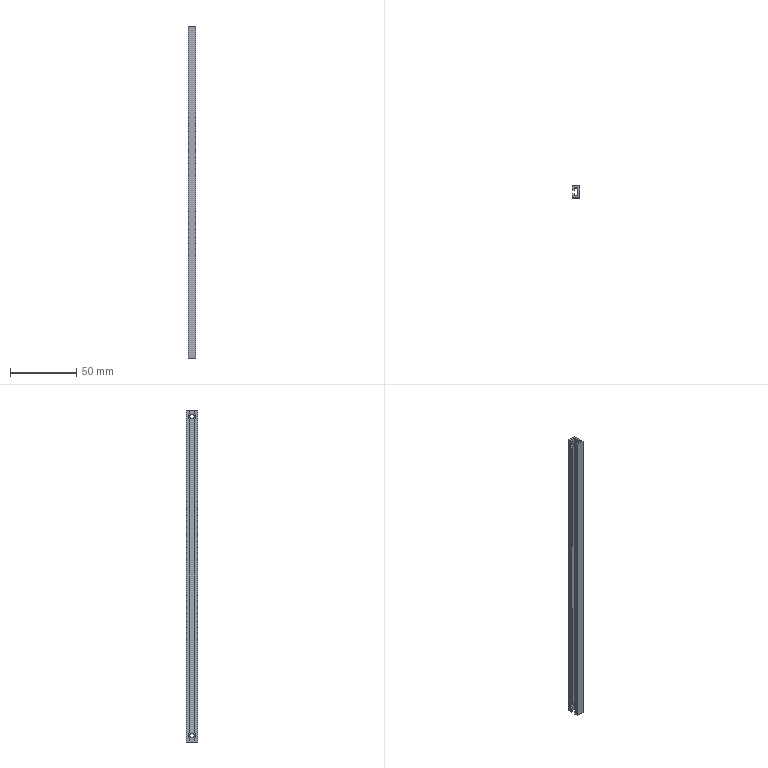Part | SolidWorks | features Extrusion 1, HoleWzd 1 | 1 solid | 34 faces | box 6 x 9 x 250 mm | volume 7894 mm3 | plane 26 | cylinder 8 | commonest cylinder face diameters 3.4 x4 6 x4
STEP:
#1=CARTESIAN_POINT('',(3.,0.,243.3));
#2=VERTEX_POINT('',#1);
#3=CARTESIAN_POINT('',(3.,0.,246.7));
#4=VERTEX_POINT('',#3);
#5=CARTESIAN_POINT('',(3.,0.,245.));
#6=DIRECTION('',(-1.,0.,0.));
#7=DIRECTION('',(0.,0.,1.));
#8=AXIS2_PLACEMENT_3D('',#5,#6,#7);
#9=CIRCLE('',#8,1.7);
#10=EDGE_CURVE('',#2,#4,#9,.T.);
#11=ORIENTED_EDGE('',*,*,#10,.F.);
#12=CARTESIAN_POINT('',(1.5,0.,243.3));
#13=VERTEX_POINT('',#12);
#14=CARTESIAN_POINT('',(-3.,0.,243.3));
#15=DIRECTION('',(-1.,0.,0.));
#16=VECTOR('',#15,1000.);
#17=LINE('',#14,#16);
#18=EDGE_CURVE('',#2,#13,#17,.T.);
#19=ORIENTED_EDGE('',*,*,#18,.T.);
#20=CARTESIAN_POINT('',(1.5,0.,246.7));
#21=VERTEX_POINT('',#20);
#22=CARTESIAN_POINT('',(1.5,0.,245.));
#23=DIRECTION('',(1.,0.,0.));
#24=DIRECTION('',(0.,0.,-1.));
#25=AXIS2_PLACEMENT_3D('',#22,#23,#24);
#26=CIRCLE('',#25,1.7);
#27=EDGE_CURVE('',#21,#13,#26,.T.);
#28=ORIENTED_EDGE('',*,*,#27,.F.);
#29=CARTESIAN_POINT('',(-3.,0.,246.7));
#30=DIRECTION('',(-1.,0.,0.));
#31=VECTOR('',#30,1000.);
#32=LINE('',#29,#31);
#33=EDGE_CURVE('',#4,#21,#32,.T.);
#34=ORIENTED_EDGE('',*,*,#33,.F.);
#35=EDGE_LOOP('',(#11,#19,#28,#34));
#36=FACE_OUTER_BOUND('',#35,.T.);
#37=CARTESIAN_POINT('',(-3.,0.,245.));
#38=DIRECTION('',(-1.,0.,0.));
#39=DIRECTION('',(0.,0.,1.));
#40=AXIS2_PLACEMENT_3D('',#37,#38,#39);
#41=CYLINDRICAL_SURFACE('',#40,1.7);
#42=ADVANCED_FACE('',(#36),#41,.F.);
#43=CARTESIAN_POINT('',(3.,0.,3.3));
#44=VERTEX_POINT('',#43);
#45=CARTESIAN_POINT('',(3.,0.,6.7));
#46=VERTEX_POINT('',#45);
#47=CARTESIAN_POINT('',(3.,0.,5.));
#48=DIRECTION('',(-1.,0.,0.));
#49=DIRECTION('',(0.,0.,1.));
#50=AXIS2_PLACEMENT_3D('',#47,#48,#49);
#51=CIRCLE('',#50,1.7);
#52=EDGE_CURVE('',#44,#46,#51,.T.);
#53=ORIENTED_EDGE('',*,*,#52,.F.);
#54=CARTESIAN_POINT('',(1.5,0.,3.3));
#55=VERTEX_POINT('',#54);
#56=CARTESIAN_POINT('',(-3.,0.,3.3));
#57=DIRECTION('',(-1.,0.,0.));
#58=VECTOR('',#57,1000.);
#59=LINE('',#56,#58);
#60=EDGE_CURVE('',#44,#55,#59,.T.);
#61=ORIENTED_EDGE('',*,*,#60,.T.);
#62=CARTESIAN_POINT('',(1.5,0.,6.7));
#63=VERTEX_POINT('',#62);
#64=CARTESIAN_POINT('',(1.5,0.,5.));
#65=DIRECTION('',(1.,0.,0.));
#66=DIRECTION('',(0.,0.,-1.));
#67=AXIS2_PLACEMENT_3D('',#64,#65,#66);
#68=CIRCLE('',#67,1.7);
#69=EDGE_CURVE('',#63,#55,#68,.T.);
#70=ORIENTED_EDGE('',*,*,#69,.F.);
#71=CARTESIAN_POINT('',(-3.,0.,6.7));
#72=DIRECTION('',(-1.,0.,0.));
#73=VECTOR('',#72,1000.);
#74=LINE('',#71,#73);
#75=EDGE_CURVE('',#46,#63,#74,.T.);
#76=ORIENTED_EDGE('',*,*,#75,.F.);
#77=EDGE_LOOP('',(#53,#61,#70,#76));
#78=FACE_OUTER_BOUND('',#77,.T.);
#79=CARTESIAN_POINT('',(-3.,0.,5.));
#80=DIRECTION('',(-1.,0.,0.));
#81=DIRECTION('',(0.,0.,1.));
#82=AXIS2_PLACEMENT_3D('',#79,#80,#81);
#83=CYLINDRICAL_SURFACE('',#82,1.7);
#84=ADVANCED_FACE('',(#78),#83,.F.);
#85=CARTESIAN_POINT('',(-1.5,1.7,250.));
#86=VERTEX_POINT('',#85);
#87=CARTESIAN_POINT('',(-1.5,1.7,247.472));
#88=VERTEX_POINT('',#87);
#89=CARTESIAN_POINT('',(-1.5,1.7,250.));
#90=DIRECTION('',(0.,0.,-1.));
#91=VECTOR('',#90,1000.);
#92=LINE('',#89,#91);
#93=EDGE_CURVE('',#86,#88,#92,.T.);
#94=ORIENTED_EDGE('',*,*,#93,.T.);
#95=CARTESIAN_POINT('',(-1.5,2.85,245.937));
#96=VERTEX_POINT('',#95);
#97=CARTESIAN_POINT('',(-1.5,0.,245.));
#98=DIRECTION('',(-1.,0.,0.));
#99=DIRECTION('',(0.,0.,1.));
#100=AXIS2_PLACEMENT_3D('',#97,#98,#99);
#101=CIRCLE('',#100,3.);
#102=EDGE_CURVE('',#88,#96,#101,.T.);
#103=ORIENTED_EDGE('',*,*,#102,.T.);
#104=CARTESIAN_POINT('',(-1.5,2.85,250.));
#105=VERTEX_POINT('',#104);
#106=CARTESIAN_POINT('',(-1.5,2.85,250.));
#107=DIRECTION('',(0.,0.,-1.));
#108=VECTOR('',#107,1000.);
#109=LINE('',#106,#108);
#110=EDGE_CURVE('',#105,#96,#109,.T.);
#111=ORIENTED_EDGE('',*,*,#110,.F.);
#112=CARTESIAN_POINT('',(-1.5,1.7,250.));
#113=DIRECTION('',(0.,1.,0.));
#114=VECTOR('',#113,1000.);
#115=LINE('',#112,#114);
#116=EDGE_CURVE('',#86,#105,#115,.T.);
#117=ORIENTED_EDGE('',*,*,#116,.F.);
#118=EDGE_LOOP('',(#94,#103,#111,#117));
#119=FACE_OUTER_BOUND('',#118,.T.);
#120=CARTESIAN_POINT('',(-1.5,1.7,250.));
#121=DIRECTION('',(-1.,0.,0.));
#122=DIRECTION('',(0.,0.,1.));
#123=AXIS2_PLACEMENT_3D('',#120,#121,#122);
#124=PLANE('',#123);
#125=ADVANCED_FACE('',(#119),#124,.F.);
#126=CARTESIAN_POINT('',(-1.5,-1.7,250.));
#127=VERTEX_POINT('',#126);
#128=CARTESIAN_POINT('',(-1.5,-1.7,247.472));
#129=VERTEX_POINT('',#128);
#130=CARTESIAN_POINT('',(-1.5,-1.7,250.));
#131=DIRECTION('',(0.,0.,-1.));
#132=VECTOR('',#131,1000.);
#133=LINE('',#130,#132);
#134=EDGE_CURVE('',#127,#129,#133,.T.);
#135=ORIENTED_EDGE('',*,*,#134,.T.);
#136=CARTESIAN_POINT('',(-3.,-1.7,247.472));
#137=VERTEX_POINT('',#136);
#138=CARTESIAN_POINT('',(-3.,-1.7,247.472));
#139=DIRECTION('',(-1.,0.,0.));
#140=VECTOR('',#139,1000.);
#141=LINE('',#138,#140);
#142=EDGE_CURVE('',#129,#137,#141,.T.);
#143=ORIENTED_EDGE('',*,*,#142,.T.);
#144=CARTESIAN_POINT('',(-3.,-1.7,250.));
#145=VERTEX_POINT('',#144);
#146=CARTESIAN_POINT('',(-3.,-1.7,250.));
#147=DIRECTION('',(0.,0.,-1.));
#148=VECTOR('',#147,1000.);
#149=LINE('',#146,#148);
#150=EDGE_CURVE('',#145,#137,#149,.T.);
#151=ORIENTED_EDGE('',*,*,#150,.F.);
#152=CARTESIAN_POINT('',(-3.,-1.7,250.));
#153=DIRECTION('',(-1.,0.,0.));
#154=VECTOR('',#153,1000.);
#155=LINE('',#152,#154);
#156=EDGE_CURVE('',#127,#145,#155,.T.);
#157=ORIENTED_EDGE('',*,*,#156,.F.);
#158=EDGE_LOOP('',(#135,#143,#151,#157));
#159=FACE_OUTER_BOUND('',#158,.T.);
#160=CARTESIAN_POINT('',(-3.,-1.7,250.));
#161=DIRECTION('',(0.,-1.,0.));
#162=DIRECTION('',(0.,0.,-1.));
#163=AXIS2_PLACEMENT_3D('',#160,#161,#162);
#164=PLANE('',#163);
#165=ADVANCED_FACE('',(#159),#164,.F.);
#166=CARTESIAN_POINT('',(-3.,1.7,247.472));
#167=VERTEX_POINT('',#166);
#168=CARTESIAN_POINT('',(-3.,1.7,242.528));
#169=VERTEX_POINT('',#168);
#170=CARTESIAN_POINT('',(-3.,0.,245.));
#171=DIRECTION('',(-1.,0.,0.));
#172=DIRECTION('',(0.,0.,1.));
#173=AXIS2_PLACEMENT_3D('',#170,#171,#172);
#174=CIRCLE('',#173,3.);
#175=EDGE_CURVE('',#167,#169,#174,.T.);
#176=ORIENTED_EDGE('',*,*,#175,.F.);
#177=CARTESIAN_POINT('',(-3.,1.7,250.));
#178=VERTEX_POINT('',#177);
#179=CARTESIAN_POINT('',(-3.,1.7,250.));
#180=DIRECTION('',(0.,0.,-1.));
#181=VECTOR('',#180,1000.);
#182=LINE('',#179,#181);
#183=EDGE_CURVE('',#178,#167,#182,.T.);
#184=ORIENTED_EDGE('',*,*,#183,.F.);
#185=CARTESIAN_POINT('',(-3.,4.5,250.));
#186=VERTEX_POINT('',#185);
#187=CARTESIAN_POINT('',(-3.,4.5,250.));
#188=DIRECTION('',(0.,-1.,0.));
#189=VECTOR('',#188,1000.);
#190=LINE('',#187,#189);
#191=EDGE_CURVE('',#186,#178,#190,.T.);
#192=ORIENTED_EDGE('',*,*,#191,.F.);
#193=CARTESIAN_POINT('',(-3.,4.5,0.));
#194=VERTEX_POINT('',#193);
#195=CARTESIAN_POINT('',(-3.,4.5,250.));
#196=DIRECTION('',(0.,0.,-1.));
#197=VECTOR('',#196,1000.);
#198=LINE('',#195,#197);
#199=EDGE_CURVE('',#186,#194,#198,.T.);
#200=ORIENTED_EDGE('',*,*,#199,.T.);
#201=CARTESIAN_POINT('',(-3.,1.7,0.));
#202=VERTEX_POINT('',#201);
#203=CARTESIAN_POINT('',(-3.,4.5,0.));
#204=DIRECTION('',(0.,-1.,0.));
#205=VECTOR('',#204,1000.);
#206=LINE('',#203,#205);
#207=EDGE_CURVE('',#194,#202,#206,.T.);
#208=ORIENTED_EDGE('',*,*,#207,.T.);
#209=CARTESIAN_POINT('',(-3.,1.7,2.528));
#210=VERTEX_POINT('',#209);
#211=CARTESIAN_POINT('',(-3.,1.7,250.));
#212=DIRECTION('',(0.,0.,-1.));
#213=VECTOR('',#212,1000.);
#214=LINE('',#211,#213);
#215=EDGE_CURVE('',#210,#202,#214,.T.);
#216=ORIENTED_EDGE('',*,*,#215,.F.);
#217=CARTESIAN_POINT('',(-3.,1.7,7.472));
#218=VERTEX_POINT('',#217);
#219=CARTESIAN_POINT('',(-3.,0.,5.));
#220=DIRECTION('',(-1.,0.,0.));
#221=DIRECTION('',(0.,0.,1.));
#222=AXIS2_PLACEMENT_3D('',#219,#220,#221);
#223=CIRCLE('',#222,3.);
#224=EDGE_CURVE('',#218,#210,#223,.T.);
#225=ORIENTED_EDGE('',*,*,#224,.F.);
#226=CARTESIAN_POINT('',(-3.,1.7,250.));
#227=DIRECTION('',(0.,0.,-1.));
#228=VECTOR('',#227,1000.);
#229=LINE('',#226,#228);
#230=EDGE_CURVE('',#169,#218,#229,.T.);
#231=ORIENTED_EDGE('',*,*,#230,.F.);
#232=EDGE_LOOP('',(#176,#184,#192,#200,#208,#216,#225,#231));
#233=FACE_OUTER_BOUND('',#232,.T.);
#234=CARTESIAN_POINT('',(-3.,4.5,250.));
#235=DIRECTION('',(1.,0.,0.));
#236=DIRECTION('',(0.,1.,0.));
#237=AXIS2_PLACEMENT_3D('',#234,#235,#236);
#238=PLANE('',#237);
#239=ADVANCED_FACE('',(#233),#238,.F.);
#240=CARTESIAN_POINT('',(-1.5,1.7,242.528));
#241=VERTEX_POINT('',#240);
#242=CARTESIAN_POINT('',(-1.5,1.7,7.472));
#243=VERTEX_POINT('',#242);
#244=CARTESIAN_POINT('',(-1.5,1.7,250.));
#245=DIRECTION('',(0.,0.,-1.));
#246=VECTOR('',#245,1000.);
#247=LINE('',#244,#246);
#248=EDGE_CURVE('',#241,#243,#247,.T.);
#249=ORIENTED_EDGE('',*,*,#248,.F.);
#250=CARTESIAN_POINT('',(-3.,1.7,242.528));
#251=DIRECTION('',(-1.,0.,0.));
#252=VECTOR('',#251,1000.);
#253=LINE('',#250,#252);
#254=EDGE_CURVE('',#241,#169,#253,.T.);
#255=ORIENTED_EDGE('',*,*,#254,.T.);
#256=ORIENTED_EDGE('',*,*,#230,.T.);
#257=CARTESIAN_POINT('',(-3.,1.7,7.472));
#258=DIRECTION('',(1.,0.,0.));
#259=VECTOR('',#258,1000.);
#260=LINE('',#257,#259);
#261=EDGE_CURVE('',#218,#243,#260,.T.);
#262=ORIENTED_EDGE('',*,*,#261,.T.);
#263=EDGE_LOOP('',(#249,#255,#256,#262));
#264=FACE_OUTER_BOUND('',#263,.T.);
#265=CARTESIAN_POINT('',(-3.,1.7,250.));
#266=DIRECTION('',(0.,1.,0.));
#267=DIRECTION('',(0.,0.,1.));
#268=AXIS2_PLACEMENT_3D('',#265,#266,#267);
#269=PLANE('',#268);
#270=ADVANCED_FACE('',(#264),#269,.F.);
#271=CARTESIAN_POINT('',(-1.5,-1.7,242.528));
#272=VERTEX_POINT('',#271);
#273=CARTESIAN_POINT('',(-1.5,-1.7,7.472));
#274=VERTEX_POINT('',#273);
#275=CARTESIAN_POINT('',(-1.5,-1.7,250.));
#276=DIRECTION('',(0.,0.,-1.));
#277=VECTOR('',#276,1000.);
#278=LINE('',#275,#277);
#279=EDGE_CURVE('',#272,#274,#278,.T.);
#280=ORIENTED_EDGE('',*,*,#279,.F.);
#281=CARTESIAN_POINT('',(-1.5,-2.85,244.063));
#282=VERTEX_POINT('',#281);
#283=CARTESIAN_POINT('',(-1.5,0.,245.));
#284=DIRECTION('',(-1.,0.,0.));
#285=DIRECTION('',(0.,0.,1.));
#286=AXIS2_PLACEMENT_3D('',#283,#284,#285);
#287=CIRCLE('',#286,3.);
#288=EDGE_CURVE('',#272,#282,#287,.T.);
#289=ORIENTED_EDGE('',*,*,#288,.T.);
#290=CARTESIAN_POINT('',(-1.5,-2.85,5.937));
#291=VERTEX_POINT('',#290);
#292=CARTESIAN_POINT('',(-1.5,-2.85,250.));
#293=DIRECTION('',(0.,0.,-1.));
#294=VECTOR('',#293,1000.);
#295=LINE('',#292,#294);
#296=EDGE_CURVE('',#282,#291,#295,.T.);
#297=ORIENTED_EDGE('',*,*,#296,.T.);
#298=CARTESIAN_POINT('',(-1.5,0.,5.));
#299=DIRECTION('',(-1.,0.,0.));
#300=DIRECTION('',(0.,0.,1.));
#301=AXIS2_PLACEMENT_3D('',#298,#299,#300);
#302=CIRCLE('',#301,3.);
#303=EDGE_CURVE('',#291,#274,#302,.T.);
#304=ORIENTED_EDGE('',*,*,#303,.T.);
#305=EDGE_LOOP('',(#280,#289,#297,#304));
#306=FACE_OUTER_BOUND('',#305,.T.);
#307=CARTESIAN_POINT('',(-1.5,-1.7,250.));
#308=DIRECTION('',(-1.,0.,0.));
#309=DIRECTION('',(0.,0.,1.));
#310=AXIS2_PLACEMENT_3D('',#307,#308,#309);
#311=PLANE('',#310);
#312=ADVANCED_FACE('',(#306),#311,.F.);
#313=CARTESIAN_POINT('',(-1.5,1.7,2.528));
#314=VERTEX_POINT('',#313);
#315=CARTESIAN_POINT('',(-1.5,1.7,0.));
#316=VERTEX_POINT('',#315);
#317=CARTESIAN_POINT('',(-1.5,1.7,250.));
#318=DIRECTION('',(0.,0.,-1.));
#319=VECTOR('',#318,1000.);
#320=LINE('',#317,#319);
#321=EDGE_CURVE('',#314,#316,#320,.T.);
#322=ORIENTED_EDGE('',*,*,#321,.F.);
#323=CARTESIAN_POINT('',(-3.,1.7,2.528));
#324=DIRECTION('',(-1.,0.,0.));
#325=VECTOR('',#324,1000.);
#326=LINE('',#323,#325);
#327=EDGE_CURVE('',#314,#210,#326,.T.);
#328=ORIENTED_EDGE('',*,*,#327,.T.);
#329=ORIENTED_EDGE('',*,*,#215,.T.);
#330=CARTESIAN_POINT('',(-3.,1.7,0.));
#331=DIRECTION('',(1.,0.,0.));
#332=VECTOR('',#331,1000.);
#333=LINE('',#330,#332);
#334=EDGE_CURVE('',#202,#316,#333,.T.);
#335=ORIENTED_EDGE('',*,*,#334,.T.);
#336=EDGE_LOOP('',(#322,#328,#329,#335));
#337=FACE_OUTER_BOUND('',#336,.T.);
#338=CARTESIAN_POINT('',(-3.,1.7,250.));
#339=DIRECTION('',(0.,1.,0.));
#340=DIRECTION('',(0.,0.,1.));
#341=AXIS2_PLACEMENT_3D('',#338,#339,#340);
#342=PLANE('',#341);
#343=ADVANCED_FACE('',(#337),#342,.F.);
#344=CARTESIAN_POINT('',(-1.5,2.85,244.063));
#345=VERTEX_POINT('',#344);
#346=CARTESIAN_POINT('',(-1.5,2.85,5.937));
#347=VERTEX_POINT('',#346);
#348=CARTESIAN_POINT('',(-1.5,2.85,250.));
#349=DIRECTION('',(0.,0.,-1.));
#350=VECTOR('',#349,1000.);
#351=LINE('',#348,#350);
#352=EDGE_CURVE('',#345,#347,#351,.T.);
#353=ORIENTED_EDGE('',*,*,#352,.F.);
#354=CARTESIAN_POINT('',(-1.5,0.,245.));
#355=DIRECTION('',(-1.,0.,0.));
#356=DIRECTION('',(0.,0.,1.));
#357=AXIS2_PLACEMENT_3D('',#354,#355,#356);
#358=CIRCLE('',#357,3.);
#359=EDGE_CURVE('',#345,#241,#358,.T.);
#360=ORIENTED_EDGE('',*,*,#359,.T.);
#361=ORIENTED_EDGE('',*,*,#248,.T.);
#362=CARTESIAN_POINT('',(-1.5,0.,5.));
#363=DIRECTION('',(-1.,0.,0.));
#364=DIRECTION('',(0.,0.,1.));
#365=AXIS2_PLACEMENT_3D('',#362,#363,#364);
#366=CIRCLE('',#365,3.);
#367=EDGE_CURVE('',#243,#347,#366,.T.);
#368=ORIENTED_EDGE('',*,*,#367,.T.);
#369=EDGE_LOOP('',(#353,#360,#361,#368));
#370=FACE_OUTER_BOUND('',#369,.T.);
#371=CARTESIAN_POINT('',(-1.5,1.7,250.));
#372=DIRECTION('',(-1.,0.,0.));
#373=DIRECTION('',(0.,0.,1.));
#374=AXIS2_PLACEMENT_3D('',#371,#372,#373);
#375=PLANE('',#374);
#376=ADVANCED_FACE('',(#370),#375,.F.);
#377=CARTESIAN_POINT('',(-1.5,-1.7,2.528));
#378=VERTEX_POINT('',#377);
#379=CARTESIAN_POINT('',(-1.5,-1.7,0.));
#380=VERTEX_POINT('',#379);
#381=CARTESIAN_POINT('',(-1.5,-1.7,250.));
#382=DIRECTION('',(0.,0.,-1.));
#383=VECTOR('',#382,1000.);
#384=LINE('',#381,#383);
#385=EDGE_CURVE('',#378,#380,#384,.T.);
#386=ORIENTED_EDGE('',*,*,#385,.F.);
#387=CARTESIAN_POINT('',(-1.5,-2.85,4.063));
#388=VERTEX_POINT('',#387);
#389=CARTESIAN_POINT('',(-1.5,0.,5.));
#390=DIRECTION('',(-1.,0.,0.));
#391=DIRECTION('',(0.,0.,1.));
#392=AXIS2_PLACEMENT_3D('',#389,#390,#391);
#393=CIRCLE('',#392,3.);
#394=EDGE_CURVE('',#378,#388,#393,.T.);
#395=ORIENTED_EDGE('',*,*,#394,.T.);
#396=CARTESIAN_POINT('',(-1.5,-2.85,0.));
#397=VERTEX_POINT('',#396);
#398=CARTESIAN_POINT('',(-1.5,-2.85,250.));
#399=DIRECTION('',(0.,0.,-1.));
#400=VECTOR('',#399,1000.);
#401=LINE('',#398,#400);
#402=EDGE_CURVE('',#388,#397,#401,.T.);
#403=ORIENTED_EDGE('',*,*,#402,.T.);
#404=CARTESIAN_POINT('',(-1.5,-1.7,0.));
#405=DIRECTION('',(0.,1.,0.));
#406=VECTOR('',#405,1000.);
#407=LINE('',#404,#406);
#408=EDGE_CURVE('',#397,#380,#407,.T.);
#409=ORIENTED_EDGE('',*,*,#408,.T.);
#410=EDGE_LOOP('',(#386,#395,#403,#409));
#411=FACE_OUTER_BOUND('',#410,.T.);
#412=CARTESIAN_POINT('',(-1.5,-1.7,250.));
#413=DIRECTION('',(-1.,0.,0.));
#414=DIRECTION('',(0.,0.,1.));
#415=AXIS2_PLACEMENT_3D('',#412,#413,#414);
#416=PLANE('',#415);
#417=ADVANCED_FACE('',(#411),#416,.F.);
#418=CARTESIAN_POINT('',(-3.,-1.7,242.528));
#419=VERTEX_POINT('',#418);
#420=CARTESIAN_POINT('',(-3.,-1.7,7.472));
#421=VERTEX_POINT('',#420);
#422=CARTESIAN_POINT('',(-3.,-1.7,250.));
#423=DIRECTION('',(0.,0.,-1.));
#424=VECTOR('',#423,1000.);
#425=LINE('',#422,#424);
#426=EDGE_CURVE('',#419,#421,#425,.T.);
#427=ORIENTED_EDGE('',*,*,#426,.F.);
#428=CARTESIAN_POINT('',(-3.,-1.7,242.528));
#429=DIRECTION('',(1.,0.,0.));
#430=VECTOR('',#429,1000.);
#431=LINE('',#428,#430);
#432=EDGE_CURVE('',#419,#272,#431,.T.);
#433=ORIENTED_EDGE('',*,*,#432,.T.);
#434=ORIENTED_EDGE('',*,*,#279,.T.);
#435=CARTESIAN_POINT('',(-3.,-1.7,7.472));
#436=DIRECTION('',(-1.,0.,0.));
#437=VECTOR('',#436,1000.);
#438=LINE('',#435,#437);
#439=EDGE_CURVE('',#274,#421,#438,.T.);
#440=ORIENTED_EDGE('',*,*,#439,.T.);
#441=EDGE_LOOP('',(#427,#433,#434,#440));
#442=FACE_OUTER_BOUND('',#441,.T.);
#443=CARTESIAN_POINT('',(-3.,-1.7,250.));
#444=DIRECTION('',(0.,-1.,0.));
#445=DIRECTION('',(0.,0.,-1.));
#446=AXIS2_PLACEMENT_3D('',#443,#444,#445);
#447=PLANE('',#446);
#448=ADVANCED_FACE('',(#442),#447,.F.);
#449=ORIENTED_EDGE('',*,*,#183,.T.);
#450=CARTESIAN_POINT('',(-3.,1.7,247.472));
#451=DIRECTION('',(1.,0.,0.));
#452=VECTOR('',#451,1000.);
#453=LINE('',#450,#452);
#454=EDGE_CURVE('',#167,#88,#453,.T.);
#455=ORIENTED_EDGE('',*,*,#454,.T.);
#456=ORIENTED_EDGE('',*,*,#93,.F.);
#457=CARTESIAN_POINT('',(-3.,1.7,250.));
#458=DIRECTION('',(1.,0.,0.));
#459=VECTOR('',#458,1000.);
#460=LINE('',#457,#459);
#461=EDGE_CURVE('',#178,#86,#460,.T.);
#462=ORIENTED_EDGE('',*,*,#461,.F.);
#463=EDGE_LOOP('',(#449,#455,#456,#462));
#464=FACE_OUTER_BOUND('',#463,.T.);
#465=CARTESIAN_POINT('',(-3.,1.7,250.));
#466=DIRECTION('',(0.,1.,0.));
#467=DIRECTION('',(0.,0.,1.));
#468=AXIS2_PLACEMENT_3D('',#465,#466,#467);
#469=PLANE('',#468);
#470=ADVANCED_FACE('',(#464),#469,.F.);
#471=CARTESIAN_POINT('',(-1.5,2.85,4.063));
#472=VERTEX_POINT('',#471);
#473=CARTESIAN_POINT('',(-1.5,2.85,0.));
#474=VERTEX_POINT('',#473);
#475=CARTESIAN_POINT('',(-1.5,2.85,250.));
#476=DIRECTION('',(0.,0.,-1.));
#477=VECTOR('',#476,1000.);
#478=LINE('',#475,#477);
#479=EDGE_CURVE('',#472,#474,#478,.T.);
#480=ORIENTED_EDGE('',*,*,#479,.F.);
#481=CARTESIAN_POINT('',(-1.5,0.,5.));
#482=DIRECTION('',(-1.,0.,0.));
#483=DIRECTION('',(0.,0.,1.));
#484=AXIS2_PLACEMENT_3D('',#481,#482,#483);
#485=CIRCLE('',#484,3.);
#486=EDGE_CURVE('',#472,#314,#485,.T.);
#487=ORIENTED_EDGE('',*,*,#486,.T.);
#488=ORIENTED_EDGE('',*,*,#321,.T.);
#489=CARTESIAN_POINT('',(-1.5,1.7,0.));
#490=DIRECTION('',(0.,1.,0.));
#491=VECTOR('',#490,1000.);
#492=LINE('',#489,#491);
#493=EDGE_CURVE('',#316,#474,#492,.T.);
#494=ORIENTED_EDGE('',*,*,#493,.T.);
#495=EDGE_LOOP('',(#480,#487,#488,#494));
#496=FACE_OUTER_BOUND('',#495,.T.);
#497=CARTESIAN_POINT('',(-1.5,1.7,250.));
#498=DIRECTION('',(-1.,0.,0.));
#499=DIRECTION('',(0.,0.,1.));
#500=AXIS2_PLACEMENT_3D('',#497,#498,#499);
#501=PLANE('',#500);
#502=ADVANCED_FACE('',(#496),#501,.F.);
#503=CARTESIAN_POINT('',(0.4,2.85,245.937));
#504=VERTEX_POINT('',#503);
#505=CARTESIAN_POINT('',(0.4,2.85,244.063));
#506=VERTEX_POINT('',#505);
#507=CARTESIAN_POINT('',(0.4,2.85,250.));
#508=DIRECTION('',(0.,0.,-1.));
#509=VECTOR('',#508,1000.);
#510=LINE('',#507,#509);
#511=EDGE_CURVE('',#504,#506,#510,.T.);
#512=ORIENTED_EDGE('',*,*,#511,.T.);
#513=CARTESIAN_POINT('',(-3.,2.85,244.063));
#514=DIRECTION('',(-1.,0.,0.));
#515=VECTOR('',#514,1000.);
#516=LINE('',#513,#515);
#517=EDGE_CURVE('',#506,#345,#516,.T.);
#518=ORIENTED_EDGE('',*,*,#517,.T.);
#519=ORIENTED_EDGE('',*,*,#352,.T.);
#520=CARTESIAN_POINT('',(0.4,2.85,5.937));
#521=VERTEX_POINT('',#520);
#522=CARTESIAN_POINT('',(-3.,2.85,5.937));
#523=DIRECTION('',(1.,0.,0.));
#524=VECTOR('',#523,1000.);
#525=LINE('',#522,#524);
#526=EDGE_CURVE('',#347,#521,#525,.T.);
#527=ORIENTED_EDGE('',*,*,#526,.T.);
#528=CARTESIAN_POINT('',(0.4,2.85,4.063));
#529=VERTEX_POINT('',#528);
#530=CARTESIAN_POINT('',(0.4,2.85,250.));
#531=DIRECTION('',(0.,0.,-1.));
#532=VECTOR('',#531,1000.);
#533=LINE('',#530,#532);
#534=EDGE_CURVE('',#521,#529,#533,.T.);
#535=ORIENTED_EDGE('',*,*,#534,.T.);
#536=CARTESIAN_POINT('',(-3.,2.85,4.063));
#537=DIRECTION('',(-1.,0.,0.));
#538=VECTOR('',#537,1000.);
#539=LINE('',#536,#538);
#540=EDGE_CURVE('',#529,#472,#539,.T.);
#541=ORIENTED_EDGE('',*,*,#540,.T.);
#542=ORIENTED_EDGE('',*,*,#479,.T.);
#543=CARTESIAN_POINT('',(1.5,2.85,0.));
#544=VERTEX_POINT('',#543);
#545=CARTESIAN_POINT('',(-1.5,2.85,0.));
#546=DIRECTION('',(1.,0.,0.));
#547=VECTOR('',#546,1000.);
#548=LINE('',#545,#547);
#549=EDGE_CURVE('',#474,#544,#548,.T.);
#550=ORIENTED_EDGE('',*,*,#549,.T.);
#551=CARTESIAN_POINT('',(1.5,2.85,250.));
#552=VERTEX_POINT('',#551);
#553=CARTESIAN_POINT('',(1.5,2.85,250.));
#554=DIRECTION('',(0.,0.,-1.));
#555=VECTOR('',#554,1000.);
#556=LINE('',#553,#555);
#557=EDGE_CURVE('',#552,#544,#556,.T.);
#558=ORIENTED_EDGE('',*,*,#557,.F.);
#559=CARTESIAN_POINT('',(-1.5,2.85,250.));
#560=DIRECTION('',(1.,0.,0.));
#561=VECTOR('',#560,1000.);
#562=LINE('',#559,#561);
#563=EDGE_CURVE('',#105,#552,#562,.T.);
#564=ORIENTED_EDGE('',*,*,#563,.F.);
#565=ORIENTED_EDGE('',*,*,#110,.T.);
#566=CARTESIAN_POINT('',(-3.,2.85,245.937));
#567=DIRECTION('',(1.,0.,0.));
#568=VECTOR('',#567,1000.);
#569=LINE('',#566,#568);
#570=EDGE_CURVE('',#96,#504,#569,.T.);
#571=ORIENTED_EDGE('',*,*,#570,.T.);
#572=EDGE_LOOP('',(#512,#518,#519,#527,#535,#541,#542,#550,#558,#564,#565,#571));
#573=FACE_OUTER_BOUND('',#572,.T.);
#574=CARTESIAN_POINT('',(-1.5,2.85,250.));
#575=DIRECTION('',(0.,1.,0.));
#576=DIRECTION('',(0.,0.,1.));
#577=AXIS2_PLACEMENT_3D('',#574,#575,#576);
#578=PLANE('',#577);
#579=ADVANCED_FACE('',(#573),#578,.F.);
#580=ORIENTED_EDGE('',*,*,#27,.T.);
#581=CARTESIAN_POINT('',(1.5,0.,245.));
#582=DIRECTION('',(1.,0.,0.));
#583=DIRECTION('',(0.,0.,-1.));
#584=AXIS2_PLACEMENT_3D('',#581,#582,#583);
#585=CIRCLE('',#584,1.7);
#586=EDGE_CURVE('',#13,#21,#585,.T.);
#587=ORIENTED_EDGE('',*,*,#586,.T.);
#588=EDGE_LOOP('',(#580,#587));
#589=FACE_BOUND('',#588,.T.);
#590=ORIENTED_EDGE('',*,*,#69,.T.);
#591=CARTESIAN_POINT('',(1.5,0.,5.));
#592=DIRECTION('',(1.,0.,0.));
#593=DIRECTION('',(0.,0.,-1.));
#594=AXIS2_PLACEMENT_3D('',#591,#592,#593);
#595=CIRCLE('',#594,1.7);
#596=EDGE_CURVE('',#55,#63,#595,.T.);
#597=ORIENTED_EDGE('',*,*,#596,.T.);
#598=EDGE_LOOP('',(#590,#597));
#599=FACE_BOUND('',#598,.T.);
#600=CARTESIAN_POINT('',(1.5,-2.85,0.));
#601=VERTEX_POINT('',#600);
#602=CARTESIAN_POINT('',(1.5,2.85,0.));
#603=DIRECTION('',(0.,-1.,0.));
#604=VECTOR('',#603,1000.);
#605=LINE('',#602,#604);
#606=EDGE_CURVE('',#544,#601,#605,.T.);
#607=ORIENTED_EDGE('',*,*,#606,.T.);
#608=CARTESIAN_POINT('',(1.5,-2.85,250.));
#609=VERTEX_POINT('',#608);
#610=CARTESIAN_POINT('',(1.5,-2.85,250.));
#611=DIRECTION('',(0.,0.,-1.));
#612=VECTOR('',#611,1000.);
#613=LINE('',#610,#612);
#614=EDGE_CURVE('',#609,#601,#613,.T.);
#615=ORIENTED_EDGE('',*,*,#614,.F.);
#616=CARTESIAN_POINT('',(1.5,2.85,250.));
#617=DIRECTION('',(0.,-1.,0.));
#618=VECTOR('',#617,1000.);
#619=LINE('',#616,#618);
#620=EDGE_CURVE('',#552,#609,#619,.T.);
#621=ORIENTED_EDGE('',*,*,#620,.F.);
#622=ORIENTED_EDGE('',*,*,#557,.T.);
#623=EDGE_LOOP('',(#607,#615,#621,#622));
#624=FACE_OUTER_BOUND('',#623,.T.);
#625=CARTESIAN_POINT('',(1.5,2.85,250.));
#626=DIRECTION('',(1.,0.,0.));
#627=DIRECTION('',(0.,0.,-1.));
#628=AXIS2_PLACEMENT_3D('',#625,#626,#627);
#629=PLANE('',#628);
#630=ADVANCED_FACE('',(#589,#599,#624),#629,.F.);
#631=CARTESIAN_POINT('',(0.4,-2.85,244.063));
#632=VERTEX_POINT('',#631);
#633=CARTESIAN_POINT('',(0.4,-2.85,245.937));
#634=VERTEX_POINT('',#633);
#635=CARTESIAN_POINT('',(0.4,-2.85,250.));
#636=DIRECTION('',(0.,0.,1.));
#637=VECTOR('',#636,1000.);
#638=LINE('',#635,#637);
#639=EDGE_CURVE('',#632,#634,#638,.T.);
#640=ORIENTED_EDGE('',*,*,#639,.T.);
#641=CARTESIAN_POINT('',(-1.5,-2.85,245.937));
#642=VERTEX_POINT('',#641);
#643=CARTESIAN_POINT('',(-3.,-2.85,245.937));
#644=DIRECTION('',(-1.,0.,0.));
#645=VECTOR('',#644,1000.);
#646=LINE('',#643,#645);
#647=EDGE_CURVE('',#634,#642,#646,.T.);
#648=ORIENTED_EDGE('',*,*,#647,.T.);
#649=CARTESIAN_POINT('',(-1.5,-2.85,250.));
#650=VERTEX_POINT('',#649);
#651=CARTESIAN_POINT('',(-1.5,-2.85,250.));
#652=DIRECTION('',(0.,0.,-1.));
#653=VECTOR('',#652,1000.);
#654=LINE('',#651,#653);
#655=EDGE_CURVE('',#650,#642,#654,.T.);
#656=ORIENTED_EDGE('',*,*,#655,.F.);
#657=CARTESIAN_POINT('',(-1.5,-2.85,250.));
#658=DIRECTION('',(-1.,0.,0.));
#659=VECTOR('',#658,1000.);
#660=LINE('',#657,#659);
#661=EDGE_CURVE('',#609,#650,#660,.T.);
#662=ORIENTED_EDGE('',*,*,#661,.F.);
#663=ORIENTED_EDGE('',*,*,#614,.T.);
#664=CARTESIAN_POINT('',(-1.5,-2.85,0.));
#665=DIRECTION('',(-1.,0.,0.));
#666=VECTOR('',#665,1000.);
#667=LINE('',#664,#666);
#668=EDGE_CURVE('',#601,#397,#667,.T.);
#669=ORIENTED_EDGE('',*,*,#668,.T.);
#670=ORIENTED_EDGE('',*,*,#402,.F.);
#671=CARTESIAN_POINT('',(0.4,-2.85,4.063));
#672=VERTEX_POINT('',#671);
#673=CARTESIAN_POINT('',(-3.,-2.85,4.063));
#674=DIRECTION('',(1.,0.,0.));
#675=VECTOR('',#674,1000.);
#676=LINE('',#673,#675);
#677=EDGE_CURVE('',#388,#672,#676,.T.);
#678=ORIENTED_EDGE('',*,*,#677,.T.);
#679=CARTESIAN_POINT('',(0.4,-2.85,5.937));
#680=VERTEX_POINT('',#679);
#681=CARTESIAN_POINT('',(0.4,-2.85,250.));
#682=DIRECTION('',(0.,0.,1.));
#683=VECTOR('',#682,1000.);
#684=LINE('',#681,#683);
#685=EDGE_CURVE('',#672,#680,#684,.T.);
#686=ORIENTED_EDGE('',*,*,#685,.T.);
#687=CARTESIAN_POINT('',(-3.,-2.85,5.937));
#688=DIRECTION('',(-1.,0.,0.));
#689=VECTOR('',#688,1000.);
#690=LINE('',#687,#689);
#691=EDGE_CURVE('',#680,#291,#690,.T.);
#692=ORIENTED_EDGE('',*,*,#691,.T.);
#693=ORIENTED_EDGE('',*,*,#296,.F.);
#694=CARTESIAN_POINT('',(-3.,-2.85,244.063));
#695=DIRECTION('',(1.,0.,0.));
#696=VECTOR('',#695,1000.);
#697=LINE('',#694,#696);
#698=EDGE_CURVE('',#282,#632,#697,.T.);
#699=ORIENTED_EDGE('',*,*,#698,.T.);
#700=EDGE_LOOP('',(#640,#648,#656,#662,#663,#669,#670,#678,#686,#692,#693,#699));
#701=FACE_OUTER_BOUND('',#700,.T.);
#702=CARTESIAN_POINT('',(-1.5,-2.85,250.));
#703=DIRECTION('',(0.,-1.,0.));
#704=DIRECTION('',(0.,0.,-1.));
#705=AXIS2_PLACEMENT_3D('',#702,#703,#704);
#706=PLANE('',#705);
#707=ADVANCED_FACE('',(#701),#706,.F.);
#708=ORIENTED_EDGE('',*,*,#655,.T.);
#709=CARTESIAN_POINT('',(-1.5,0.,245.));
#710=DIRECTION('',(-1.,0.,0.));
#711=DIRECTION('',(0.,0.,1.));
#712=AXIS2_PLACEMENT_3D('',#709,#710,#711);
#713=CIRCLE('',#712,3.);
#714=EDGE_CURVE('',#642,#129,#713,.T.);
#715=ORIENTED_EDGE('',*,*,#714,.T.);
#716=ORIENTED_EDGE('',*,*,#134,.F.);
#717=CARTESIAN_POINT('',(-1.5,-1.7,250.));
#718=DIRECTION('',(0.,1.,0.));
#719=VECTOR('',#718,1000.);
#720=LINE('',#717,#719);
#721=EDGE_CURVE('',#650,#127,#720,.T.);
#722=ORIENTED_EDGE('',*,*,#721,.F.);
#723=EDGE_LOOP('',(#708,#715,#716,#722));
#724=FACE_OUTER_BOUND('',#723,.T.);
#725=CARTESIAN_POINT('',(-1.5,-1.7,250.));
#726=DIRECTION('',(-1.,0.,0.));
#727=DIRECTION('',(0.,0.,1.));
#728=AXIS2_PLACEMENT_3D('',#725,#726,#727);
#729=PLANE('',#728);
#730=ADVANCED_FACE('',(#724),#729,.F.);
#731=CARTESIAN_POINT('',(-3.,-1.7,2.528));
#732=VERTEX_POINT('',#731);
#733=CARTESIAN_POINT('',(-3.,-1.7,0.));
#734=VERTEX_POINT('',#733);
#735=CARTESIAN_POINT('',(-3.,-1.7,250.));
#736=DIRECTION('',(0.,0.,-1.));
#737=VECTOR('',#736,1000.);
#738=LINE('',#735,#737);
#739=EDGE_CURVE('',#732,#734,#738,.T.);
#740=ORIENTED_EDGE('',*,*,#739,.F.);
#741=CARTESIAN_POINT('',(-3.,-1.7,2.528));
#742=DIRECTION('',(1.,0.,0.));
#743=VECTOR('',#742,1000.);
#744=LINE('',#741,#743);
#745=EDGE_CURVE('',#732,#378,#744,.T.);
#746=ORIENTED_EDGE('',*,*,#745,.T.);
#747=ORIENTED_EDGE('',*,*,#385,.T.);
#748=CARTESIAN_POINT('',(-3.,-1.7,0.));
#749=DIRECTION('',(-1.,0.,0.));
#750=VECTOR('',#749,1000.);
#751=LINE('',#748,#750);
#752=EDGE_CURVE('',#380,#734,#751,.T.);
#753=ORIENTED_EDGE('',*,*,#752,.T.);
#754=EDGE_LOOP('',(#740,#746,#747,#753));
#755=FACE_OUTER_BOUND('',#754,.T.);
#756=CARTESIAN_POINT('',(-3.,-1.7,250.));
#757=DIRECTION('',(0.,-1.,0.));
#758=DIRECTION('',(0.,0.,-1.));
#759=AXIS2_PLACEMENT_3D('',#756,#757,#758);
#760=PLANE('',#759);
#761=ADVANCED_FACE('',(#755),#760,.F.);
#762=ORIENTED_EDGE('',*,*,#150,.T.);
#763=CARTESIAN_POINT('',(-3.,0.,245.));
#764=DIRECTION('',(1.,0.,0.));
#765=DIRECTION('',(0.,0.,-1.));
#766=AXIS2_PLACEMENT_3D('',#763,#764,#765);
#767=CIRCLE('',#766,3.);
#768=EDGE_CURVE('',#137,#419,#767,.T.);
#769=ORIENTED_EDGE('',*,*,#768,.T.);
#770=ORIENTED_EDGE('',*,*,#426,.T.);
#771=CARTESIAN_POINT('',(-3.,0.,5.));
#772=DIRECTION('',(1.,0.,0.));
#773=DIRECTION('',(0.,0.,-1.));
#774=AXIS2_PLACEMENT_3D('',#771,#772,#773);
#775=CIRCLE('',#774,3.);
#776=EDGE_CURVE('',#421,#732,#775,.T.);
#777=ORIENTED_EDGE('',*,*,#776,.T.);
#778=ORIENTED_EDGE('',*,*,#739,.T.);
#779=CARTESIAN_POINT('',(-3.,-4.5,0.));
#780=VERTEX_POINT('',#779);
#781=CARTESIAN_POINT('',(-3.,-1.7,0.));
#782=DIRECTION('',(0.,-1.,0.));
#783=VECTOR('',#782,1000.);
#784=LINE('',#781,#783);
#785=EDGE_CURVE('',#734,#780,#784,.T.);
#786=ORIENTED_EDGE('',*,*,#785,.T.);
#787=CARTESIAN_POINT('',(-3.,-4.5,250.));
#788=VERTEX_POINT('',#787);
#789=CARTESIAN_POINT('',(-3.,-4.5,250.));
#790=DIRECTION('',(0.,0.,-1.));
#791=VECTOR('',#790,1000.);
#792=LINE('',#789,#791);
#793=EDGE_CURVE('',#788,#780,#792,.T.);
#794=ORIENTED_EDGE('',*,*,#793,.F.);
#795=CARTESIAN_POINT('',(-3.,-1.7,250.));
#796=DIRECTION('',(0.,-1.,0.));
#797=VECTOR('',#796,1000.);
#798=LINE('',#795,#797);
#799=EDGE_CURVE('',#145,#788,#798,.T.);
#800=ORIENTED_EDGE('',*,*,#799,.F.);
#801=EDGE_LOOP('',(#762,#769,#770,#777,#778,#786,#794,#800));
#802=FACE_OUTER_BOUND('',#801,.T.);
#803=CARTESIAN_POINT('',(-3.,-1.7,250.));
#804=DIRECTION('',(1.,0.,0.));
#805=DIRECTION('',(0.,0.,-1.));
#806=AXIS2_PLACEMENT_3D('',#803,#804,#805);
#807=PLANE('',#806);
#808=ADVANCED_FACE('',(#802),#807,.F.);
#809=CARTESIAN_POINT('',(3.,-4.5,0.));
#810=VERTEX_POINT('',#809);
#811=CARTESIAN_POINT('',(-3.,-4.5,0.));
#812=DIRECTION('',(1.,0.,0.));
#813=VECTOR('',#812,1000.);
#814=LINE('',#811,#813);
#815=EDGE_CURVE('',#780,#810,#814,.T.);
#816=ORIENTED_EDGE('',*,*,#815,.T.);
#817=CARTESIAN_POINT('',(3.,-4.5,250.));
#818=VERTEX_POINT('',#817);
#819=CARTESIAN_POINT('',(3.,-4.5,250.));
#820=DIRECTION('',(0.,0.,-1.));
#821=VECTOR('',#820,1000.);
#822=LINE('',#819,#821);
#823=EDGE_CURVE('',#818,#810,#822,.T.);
#824=ORIENTED_EDGE('',*,*,#823,.F.);
#825=CARTESIAN_POINT('',(-3.,-4.5,250.));
#826=DIRECTION('',(1.,0.,0.));
#827=VECTOR('',#826,1000.);
#828=LINE('',#825,#827);
#829=EDGE_CURVE('',#788,#818,#828,.T.);
#830=ORIENTED_EDGE('',*,*,#829,.F.);
#831=ORIENTED_EDGE('',*,*,#793,.T.);
#832=EDGE_LOOP('',(#816,#824,#830,#831));
#833=FACE_OUTER_BOUND('',#832,.T.);
#834=CARTESIAN_POINT('',(-3.,-4.5,250.));
#835=DIRECTION('',(0.,1.,0.));
#836=DIRECTION('',(-1.,0.,0.));
#837=AXIS2_PLACEMENT_3D('',#834,#835,#836);
#838=PLANE('',#837);
#839=ADVANCED_FACE('',(#833),#838,.F.);
#840=CARTESIAN_POINT('',(3.,0.,245.));
#841=DIRECTION('',(-1.,0.,0.));
#842=DIRECTION('',(0.,0.,1.));
#843=AXIS2_PLACEMENT_3D('',#840,#841,#842);
#844=CIRCLE('',#843,1.7);
#845=EDGE_CURVE('',#4,#2,#844,.T.);
#846=ORIENTED_EDGE('',*,*,#845,.T.);
#847=ORIENTED_EDGE('',*,*,#10,.T.);
#848=EDGE_LOOP('',(#846,#847));
#849=FACE_BOUND('',#848,.T.);
#850=CARTESIAN_POINT('',(3.,0.,5.));
#851=DIRECTION('',(-1.,0.,0.));
#852=DIRECTION('',(0.,0.,1.));
#853=AXIS2_PLACEMENT_3D('',#850,#851,#852);
#854=CIRCLE('',#853,1.7);
#855=EDGE_CURVE('',#46,#44,#854,.T.);
#856=ORIENTED_EDGE('',*,*,#855,.T.);
#857=ORIENTED_EDGE('',*,*,#52,.T.);
#858=EDGE_LOOP('',(#856,#857));
#859=FACE_BOUND('',#858,.T.);
#860=CARTESIAN_POINT('',(3.,4.5,0.));
#861=VERTEX_POINT('',#860);
#862=CARTESIAN_POINT('',(3.,4.5,0.));
#863=DIRECTION('',(0.,1.,0.));
#864=VECTOR('',#863,1000.);
#865=LINE('',#862,#864);
#866=EDGE_CURVE('',#810,#861,#865,.T.);
#867=ORIENTED_EDGE('',*,*,#866,.T.);
#868=CARTESIAN_POINT('',(3.,4.5,250.));
#869=VERTEX_POINT('',#868);
#870=CARTESIAN_POINT('',(3.,4.5,250.));
#871=DIRECTION('',(0.,0.,-1.));
#872=VECTOR('',#871,1000.);
#873=LINE('',#870,#872);
#874=EDGE_CURVE('',#869,#861,#873,.T.);
#875=ORIENTED_EDGE('',*,*,#874,.F.);
#876=CARTESIAN_POINT('',(3.,4.5,250.));
#877=DIRECTION('',(0.,1.,0.));
#878=VECTOR('',#877,1000.);
#879=LINE('',#876,#878);
#880=EDGE_CURVE('',#818,#869,#879,.T.);
#881=ORIENTED_EDGE('',*,*,#880,.F.);
#882=ORIENTED_EDGE('',*,*,#823,.T.);
#883=EDGE_LOOP('',(#867,#875,#881,#882));
#884=FACE_OUTER_BOUND('',#883,.T.);
#885=CARTESIAN_POINT('',(3.,4.5,250.));
#886=DIRECTION('',(-1.,0.,0.));
#887=DIRECTION('',(0.,0.,1.));
#888=AXIS2_PLACEMENT_3D('',#885,#886,#887);
#889=PLANE('',#888);
#890=ADVANCED_FACE('',(#849,#859,#884),#889,.F.);
#891=CARTESIAN_POINT('',(-3.,4.5,0.));
#892=DIRECTION('',(-1.,0.,0.));
#893=VECTOR('',#892,1000.);
#894=LINE('',#891,#893);
#895=EDGE_CURVE('',#861,#194,#894,.T.);
#896=ORIENTED_EDGE('',*,*,#895,.T.);
#897=ORIENTED_EDGE('',*,*,#199,.F.);
#898=CARTESIAN_POINT('',(-3.,4.5,250.));
#899=DIRECTION('',(-1.,0.,0.));
#900=VECTOR('',#899,1000.);
#901=LINE('',#898,#900);
#902=EDGE_CURVE('',#869,#186,#901,.T.);
#903=ORIENTED_EDGE('',*,*,#902,.F.);
#904=ORIENTED_EDGE('',*,*,#874,.T.);
#905=EDGE_LOOP('',(#896,#897,#903,#904));
#906=FACE_OUTER_BOUND('',#905,.T.);
#907=CARTESIAN_POINT('',(-3.,4.5,250.));
#908=DIRECTION('',(0.,-1.,0.));
#909=DIRECTION('',(0.,0.,-1.));
#910=AXIS2_PLACEMENT_3D('',#907,#908,#909);
#911=PLANE('',#910);
#912=ADVANCED_FACE('',(#906),#911,.F.);
#913=ORIENTED_EDGE('',*,*,#191,.T.);
#914=ORIENTED_EDGE('',*,*,#461,.T.);
#915=ORIENTED_EDGE('',*,*,#116,.T.);
#916=ORIENTED_EDGE('',*,*,#563,.T.);
#917=ORIENTED_EDGE('',*,*,#620,.T.);
#918=ORIENTED_EDGE('',*,*,#661,.T.);
#919=ORIENTED_EDGE('',*,*,#721,.T.);
#920=ORIENTED_EDGE('',*,*,#156,.T.);
#921=ORIENTED_EDGE('',*,*,#799,.T.);
#922=ORIENTED_EDGE('',*,*,#829,.T.);
#923=ORIENTED_EDGE('',*,*,#880,.T.);
#924=ORIENTED_EDGE('',*,*,#902,.T.);
#925=EDGE_LOOP('',(#913,#914,#915,#916,#917,#918,#919,#920,#921,#922,#923,#924));
#926=FACE_OUTER_BOUND('',#925,.T.);
#927=CARTESIAN_POINT('',(-3.,1.7,250.));
#928=DIRECTION('',(0.,0.,1.));
#929=DIRECTION('',(1.,0.,0.));
#930=AXIS2_PLACEMENT_3D('',#927,#928,#929);
#931=PLANE('',#930);
#932=ADVANCED_FACE('',(#926),#931,.T.);
#933=ORIENTED_EDGE('',*,*,#207,.F.);
#934=ORIENTED_EDGE('',*,*,#895,.F.);
#935=ORIENTED_EDGE('',*,*,#866,.F.);
#936=ORIENTED_EDGE('',*,*,#815,.F.);
#937=ORIENTED_EDGE('',*,*,#785,.F.);
#938=ORIENTED_EDGE('',*,*,#752,.F.);
#939=ORIENTED_EDGE('',*,*,#408,.F.);
#940=ORIENTED_EDGE('',*,*,#668,.F.);
#941=ORIENTED_EDGE('',*,*,#606,.F.);
#942=ORIENTED_EDGE('',*,*,#549,.F.);
#943=ORIENTED_EDGE('',*,*,#493,.F.);
#944=ORIENTED_EDGE('',*,*,#334,.F.);
#945=EDGE_LOOP('',(#933,#934,#935,#936,#937,#938,#939,#940,#941,#942,#943,#944));
#946=FACE_OUTER_BOUND('',#945,.T.);
#947=CARTESIAN_POINT('',(-3.,1.7,0.));
#948=DIRECTION('',(0.,0.,1.));
#949=DIRECTION('',(1.,0.,0.));
#950=AXIS2_PLACEMENT_3D('',#947,#948,#949);
#951=PLANE('',#950);
#952=ADVANCED_FACE('',(#946),#951,.F.);
#953=ORIENTED_EDGE('',*,*,#60,.F.);
#954=ORIENTED_EDGE('',*,*,#855,.F.);
#955=ORIENTED_EDGE('',*,*,#75,.T.);
#956=ORIENTED_EDGE('',*,*,#596,.F.);
#957=EDGE_LOOP('',(#953,#954,#955,#956));
#958=FACE_OUTER_BOUND('',#957,.T.);
#959=CARTESIAN_POINT('',(-3.,0.,5.));
#960=DIRECTION('',(-1.,0.,0.));
#961=DIRECTION('',(0.,0.,1.));
#962=AXIS2_PLACEMENT_3D('',#959,#960,#961);
#963=CYLINDRICAL_SURFACE('',#962,1.7);
#964=ADVANCED_FACE('',(#958),#963,.F.);
#965=CARTESIAN_POINT('',(0.4,0.,5.));
#966=DIRECTION('',(-1.,0.,0.));
#967=DIRECTION('',(0.,0.,1.));
#968=AXIS2_PLACEMENT_3D('',#965,#966,#967);
#969=CIRCLE('',#968,3.);
#970=EDGE_CURVE('',#672,#680,#969,.T.);
#971=ORIENTED_EDGE('',*,*,#970,.F.);
#972=ORIENTED_EDGE('',*,*,#677,.F.);
#973=ORIENTED_EDGE('',*,*,#394,.F.);
#974=ORIENTED_EDGE('',*,*,#745,.F.);
#975=ORIENTED_EDGE('',*,*,#776,.F.);
#976=ORIENTED_EDGE('',*,*,#439,.F.);
#977=ORIENTED_EDGE('',*,*,#303,.F.);
#978=ORIENTED_EDGE('',*,*,#691,.F.);
#979=EDGE_LOOP('',(#971,#972,#973,#974,#975,#976,#977,#978));
#980=FACE_OUTER_BOUND('',#979,.T.);
#981=CARTESIAN_POINT('',(-3.,0.,5.));
#982=DIRECTION('',(-1.,0.,0.));
#983=DIRECTION('',(0.,0.,1.));
#984=AXIS2_PLACEMENT_3D('',#981,#982,#983);
#985=CYLINDRICAL_SURFACE('',#984,3.);
#986=ADVANCED_FACE('',(#980),#985,.F.);
#987=ORIENTED_EDGE('',*,*,#970,.T.);
#988=ORIENTED_EDGE('',*,*,#685,.F.);
#989=EDGE_LOOP('',(#987,#988));
#990=FACE_OUTER_BOUND('',#989,.T.);
#991=CARTESIAN_POINT('',(0.4,1.7,5.));
#992=DIRECTION('',(1.,0.,0.));
#993=DIRECTION('',(0.,0.,-1.));
#994=AXIS2_PLACEMENT_3D('',#991,#992,#993);
#995=PLANE('',#994);
#996=ADVANCED_FACE('',(#990),#995,.F.);
#997=CARTESIAN_POINT('',(0.4,0.,5.));
#998=DIRECTION('',(-1.,0.,0.));
#999=DIRECTION('',(0.,0.,1.));
#1000=AXIS2_PLACEMENT_3D('',#997,#998,#999);
#1001=CIRCLE('',#1000,3.);
#1002=EDGE_CURVE('',#521,#529,#1001,.T.);
#1003=ORIENTED_EDGE('',*,*,#1002,.T.);
#1004=ORIENTED_EDGE('',*,*,#534,.F.);
#1005=EDGE_LOOP('',(#1003,#1004));
#1006=FACE_OUTER_BOUND('',#1005,.T.);
#1007=CARTESIAN_POINT('',(0.4,1.7,5.));
#1008=DIRECTION('',(1.,0.,0.));
#1009=DIRECTION('',(0.,0.,-1.));
#1010=AXIS2_PLACEMENT_3D('',#1007,#1008,#1009);
#1011=PLANE('',#1010);
#1012=ADVANCED_FACE('',(#1006),#1011,.F.);
#1013=ORIENTED_EDGE('',*,*,#486,.F.);
#1014=ORIENTED_EDGE('',*,*,#540,.F.);
#1015=ORIENTED_EDGE('',*,*,#1002,.F.);
#1016=ORIENTED_EDGE('',*,*,#526,.F.);
#1017=ORIENTED_EDGE('',*,*,#367,.F.);
#1018=ORIENTED_EDGE('',*,*,#261,.F.);
#1019=ORIENTED_EDGE('',*,*,#224,.T.);
#1020=ORIENTED_EDGE('',*,*,#327,.F.);
#1021=EDGE_LOOP('',(#1013,#1014,#1015,#1016,#1017,#1018,#1019,#1020));
#1022=FACE_OUTER_BOUND('',#1021,.T.);
#1023=CARTESIAN_POINT('',(-3.,0.,5.));
#1024=DIRECTION('',(-1.,0.,0.));
#1025=DIRECTION('',(0.,0.,1.));
#1026=AXIS2_PLACEMENT_3D('',#1023,#1024,#1025);
#1027=CYLINDRICAL_SURFACE('',#1026,3.);
#1028=ADVANCED_FACE('',(#1022),#1027,.F.);
#1029=ORIENTED_EDGE('',*,*,#18,.F.);
#1030=ORIENTED_EDGE('',*,*,#845,.F.);
#1031=ORIENTED_EDGE('',*,*,#33,.T.);
#1032=ORIENTED_EDGE('',*,*,#586,.F.);
#1033=EDGE_LOOP('',(#1029,#1030,#1031,#1032));
#1034=FACE_OUTER_BOUND('',#1033,.T.);
#1035=CARTESIAN_POINT('',(-3.,0.,245.));
#1036=DIRECTION('',(-1.,0.,0.));
#1037=DIRECTION('',(0.,0.,1.));
#1038=AXIS2_PLACEMENT_3D('',#1035,#1036,#1037);
#1039=CYLINDRICAL_SURFACE('',#1038,1.7);
#1040=ADVANCED_FACE('',(#1034),#1039,.F.);
#1041=ORIENTED_EDGE('',*,*,#768,.F.);
#1042=ORIENTED_EDGE('',*,*,#142,.F.);
#1043=ORIENTED_EDGE('',*,*,#714,.F.);
#1044=ORIENTED_EDGE('',*,*,#647,.F.);
#1045=CARTESIAN_POINT('',(0.4,0.,245.));
#1046=DIRECTION('',(-1.,0.,0.));
#1047=DIRECTION('',(0.,0.,1.));
#1048=AXIS2_PLACEMENT_3D('',#1045,#1046,#1047);
#1049=CIRCLE('',#1048,3.);
#1050=EDGE_CURVE('',#632,#634,#1049,.T.);
#1051=ORIENTED_EDGE('',*,*,#1050,.F.);
#1052=ORIENTED_EDGE('',*,*,#698,.F.);
#1053=ORIENTED_EDGE('',*,*,#288,.F.);
#1054=ORIENTED_EDGE('',*,*,#432,.F.);
#1055=EDGE_LOOP('',(#1041,#1042,#1043,#1044,#1051,#1052,#1053,#1054));
#1056=FACE_OUTER_BOUND('',#1055,.T.);
#1057=CARTESIAN_POINT('',(-3.,0.,245.));
#1058=DIRECTION('',(-1.,0.,0.));
#1059=DIRECTION('',(0.,0.,1.));
#1060=AXIS2_PLACEMENT_3D('',#1057,#1058,#1059);
#1061=CYLINDRICAL_SURFACE('',#1060,3.);
#1062=ADVANCED_FACE('',(#1056),#1061,.F.);
#1063=ORIENTED_EDGE('',*,*,#1050,.T.);
#1064=ORIENTED_EDGE('',*,*,#639,.F.);
#1065=EDGE_LOOP('',(#1063,#1064));
#1066=FACE_OUTER_BOUND('',#1065,.T.);
#1067=CARTESIAN_POINT('',(0.4,1.7,245.));
#1068=DIRECTION('',(1.,0.,0.));
#1069=DIRECTION('',(0.,0.,-1.));
#1070=AXIS2_PLACEMENT_3D('',#1067,#1068,#1069);
#1071=PLANE('',#1070);
#1072=ADVANCED_FACE('',(#1066),#1071,.F.);
#1073=CARTESIAN_POINT('',(0.4,0.,245.));
#1074=DIRECTION('',(-1.,0.,0.));
#1075=DIRECTION('',(0.,0.,1.));
#1076=AXIS2_PLACEMENT_3D('',#1073,#1074,#1075);
#1077=CIRCLE('',#1076,3.);
#1078=EDGE_CURVE('',#504,#506,#1077,.T.);
#1079=ORIENTED_EDGE('',*,*,#1078,.T.);
#1080=ORIENTED_EDGE('',*,*,#511,.F.);
#1081=EDGE_LOOP('',(#1079,#1080));
#1082=FACE_OUTER_BOUND('',#1081,.T.);
#1083=CARTESIAN_POINT('',(0.4,1.7,245.));
#1084=DIRECTION('',(1.,0.,0.));
#1085=DIRECTION('',(0.,0.,-1.));
#1086=AXIS2_PLACEMENT_3D('',#1083,#1084,#1085);
#1087=PLANE('',#1086);
#1088=ADVANCED_FACE('',(#1082),#1087,.F.);
#1089=ORIENTED_EDGE('',*,*,#359,.F.);
#1090=ORIENTED_EDGE('',*,*,#517,.F.);
#1091=ORIENTED_EDGE('',*,*,#1078,.F.);
#1092=ORIENTED_EDGE('',*,*,#570,.F.);
#1093=ORIENTED_EDGE('',*,*,#102,.F.);
#1094=ORIENTED_EDGE('',*,*,#454,.F.);
#1095=ORIENTED_EDGE('',*,*,#175,.T.);
#1096=ORIENTED_EDGE('',*,*,#254,.F.);
#1097=EDGE_LOOP('',(#1089,#1090,#1091,#1092,#1093,#1094,#1095,#1096));
#1098=FACE_OUTER_BOUND('',#1097,.T.);
#1099=CARTESIAN_POINT('',(-3.,0.,245.));
#1100=DIRECTION('',(-1.,0.,0.));
#1101=DIRECTION('',(0.,0.,1.));
#1102=AXIS2_PLACEMENT_3D('',#1099,#1100,#1101);
#1103=CYLINDRICAL_SURFACE('',#1102,3.);
#1104=ADVANCED_FACE('',(#1098),#1103,.F.);
#1105=CLOSED_SHELL('',(#42,#84,#125,#165,#239,#270,#312,#343,#376,#417,#448,#470,#502,#579,#630,#707,#730,#761,#808,#839,#890,#912,#932,#952,#964,#986,#996,#1012,#1028,#1040,#1062,#1072,#1088,#1104));
#1106=MANIFOLD_SOLID_BREP('',#1105);
#1107=CARTESIAN_POINT('',(0.,0.,0.));
#1108=DIRECTION('',(0.,0.,1.));
#1109=DIRECTION('',(1.,0.,0.));
#1110=AXIS2_PLACEMENT_3D('',#1107,#1108,#1109);
#1111=(LENGTH_UNIT()NAMED_UNIT(*)SI_UNIT(.MILLI.,.METRE.));
#1112=UNCERTAINTY_MEASURE_WITH_UNIT(LENGTH_MEASURE(0.00001),#1111,'','');
#1113=(NAMED_UNIT(*)PLANE_ANGLE_UNIT()SI_UNIT($,.RADIAN.));
#1114=(NAMED_UNIT(*)SI_UNIT($,.STERADIAN.)SOLID_ANGLE_UNIT());
#1115=(GEOMETRIC_REPRESENTATION_CONTEXT(3)GLOBAL_UNCERTAINTY_ASSIGNED_CONTEXT((#1112))GLOBAL_UNIT_ASSIGNED_CONTEXT((#1111,#1113,#1114))REPRESENTATION_CONTEXT('',''));
#1116=ADVANCED_BREP_SHAPE_REPRESENTATION('',(#1106,#1110),#1115);